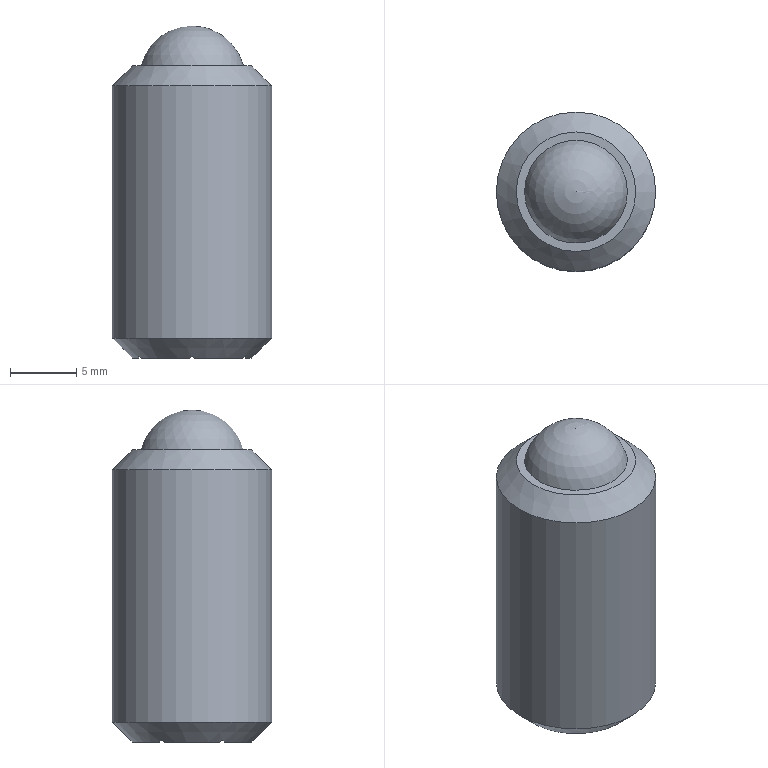Part | NX | features BZM12.00 2 | 1 solid | 18 faces | box 12 x 12 x 25 mm | volume 2052 mm3 | plane 14 | cone 2 | cylinder 1 | sphere 1 | commonest cylinder face diameters 12 x1
STEP:
#1=CARTESIAN_POINT('',(-101.,-82.938,-72.));
#2=VERTEX_POINT('',#1);
#3=CARTESIAN_POINT('',(-101.,-87.062,-72.));
#4=VERTEX_POINT('',#3);
#5=CARTESIAN_POINT('',(-101.,-82.691,-72.));
#6=DIRECTION('',(0.,-1.,0.));
#7=VECTOR('',#6,1000.);
#8=LINE('',#5,#7);
#9=EDGE_CURVE('',#2,#4,#8,.T.);
#10=ORIENTED_EDGE('',*,*,#9,.F.);
#11=CARTESIAN_POINT('',(-105.,-85.,-72.));
#12=DIRECTION('',(0.,0.,1.));
#13=DIRECTION('',(-1.,0.,0.));
#14=AXIS2_PLACEMENT_3D('',#11,#12,#13);
#15=CIRCLE('',#14,4.5);
#16=EDGE_CURVE('',#4,#2,#15,.T.);
#17=ORIENTED_EDGE('',*,*,#16,.F.);
#18=EDGE_LOOP('',(#10,#17));
#19=FACE_BOUND('',#18,.T.);
#20=CARTESIAN_POINT('',(-105.,-85.,-72.));
#21=DIRECTION('',(0.,0.,-1.));
#22=DIRECTION('',(-1.,0.,0.));
#23=AXIS2_PLACEMENT_3D('',#20,#21,#22);
#24=PLANE('',#23);
#25=ADVANCED_FACE('',(#19),#24,.T.);
#26=CARTESIAN_POINT('',(-104.785,-80.505,-72.));
#27=VERTEX_POINT('',#26);
#28=CARTESIAN_POINT('',(-101.215,-82.567,-72.));
#29=VERTEX_POINT('',#28);
#30=CARTESIAN_POINT('',(-105.,-80.381,-72.));
#31=DIRECTION('',(0.866,-0.5,0.));
#32=VECTOR('',#31,1000.);
#33=LINE('',#30,#32);
#34=EDGE_CURVE('',#27,#29,#33,.T.);
#35=ORIENTED_EDGE('',*,*,#34,.F.);
#36=CARTESIAN_POINT('',(-105.,-85.,-72.));
#37=DIRECTION('',(0.,0.,1.));
#38=DIRECTION('',(-1.,0.,0.));
#39=AXIS2_PLACEMENT_3D('',#36,#37,#38);
#40=CIRCLE('',#39,4.5);
#41=EDGE_CURVE('',#29,#27,#40,.T.);
#42=ORIENTED_EDGE('',*,*,#41,.F.);
#43=EDGE_LOOP('',(#35,#42));
#44=FACE_BOUND('',#43,.T.);
#45=CARTESIAN_POINT('',(-105.,-85.,-72.));
#46=DIRECTION('',(0.,0.,-1.));
#47=DIRECTION('',(-1.,0.,0.));
#48=AXIS2_PLACEMENT_3D('',#45,#46,#47);
#49=PLANE('',#48);
#50=ADVANCED_FACE('',(#44),#49,.T.);
#51=CARTESIAN_POINT('',(-108.785,-82.567,-72.));
#52=VERTEX_POINT('',#51);
#53=CARTESIAN_POINT('',(-105.215,-80.505,-72.));
#54=VERTEX_POINT('',#53);
#55=CARTESIAN_POINT('',(-109.,-82.691,-72.));
#56=DIRECTION('',(0.866,0.5,0.));
#57=VECTOR('',#56,1000.);
#58=LINE('',#55,#57);
#59=EDGE_CURVE('',#52,#54,#58,.T.);
#60=ORIENTED_EDGE('',*,*,#59,.F.);
#61=CARTESIAN_POINT('',(-105.,-85.,-72.));
#62=DIRECTION('',(0.,0.,1.));
#63=DIRECTION('',(-1.,0.,0.));
#64=AXIS2_PLACEMENT_3D('',#61,#62,#63);
#65=CIRCLE('',#64,4.5);
#66=EDGE_CURVE('',#54,#52,#65,.T.);
#67=ORIENTED_EDGE('',*,*,#66,.F.);
#68=EDGE_LOOP('',(#60,#67));
#69=FACE_BOUND('',#68,.T.);
#70=CARTESIAN_POINT('',(-105.,-85.,-72.));
#71=DIRECTION('',(0.,0.,-1.));
#72=DIRECTION('',(-1.,0.,0.));
#73=AXIS2_PLACEMENT_3D('',#70,#71,#72);
#74=PLANE('',#73);
#75=ADVANCED_FACE('',(#69),#74,.T.);
#76=CARTESIAN_POINT('',(-109.,-87.062,-72.));
#77=VERTEX_POINT('',#76);
#78=CARTESIAN_POINT('',(-109.,-82.938,-72.));
#79=VERTEX_POINT('',#78);
#80=CARTESIAN_POINT('',(-109.,-87.309,-72.));
#81=DIRECTION('',(0.,1.,0.));
#82=VECTOR('',#81,1000.);
#83=LINE('',#80,#82);
#84=EDGE_CURVE('',#77,#79,#83,.T.);
#85=ORIENTED_EDGE('',*,*,#84,.F.);
#86=CARTESIAN_POINT('',(-105.,-85.,-72.));
#87=DIRECTION('',(0.,0.,1.));
#88=DIRECTION('',(-1.,0.,0.));
#89=AXIS2_PLACEMENT_3D('',#86,#87,#88);
#90=CIRCLE('',#89,4.5);
#91=EDGE_CURVE('',#79,#77,#90,.T.);
#92=ORIENTED_EDGE('',*,*,#91,.F.);
#93=EDGE_LOOP('',(#85,#92));
#94=FACE_BOUND('',#93,.T.);
#95=CARTESIAN_POINT('',(-105.,-85.,-72.));
#96=DIRECTION('',(0.,0.,-1.));
#97=DIRECTION('',(-1.,0.,0.));
#98=AXIS2_PLACEMENT_3D('',#95,#96,#97);
#99=PLANE('',#98);
#100=ADVANCED_FACE('',(#94),#99,.T.);
#101=CARTESIAN_POINT('',(-105.215,-89.495,-72.));
#102=VERTEX_POINT('',#101);
#103=CARTESIAN_POINT('',(-108.785,-87.433,-72.));
#104=VERTEX_POINT('',#103);
#105=CARTESIAN_POINT('',(-105.,-89.619,-72.));
#106=DIRECTION('',(-0.866,0.5,0.));
#107=VECTOR('',#106,1000.);
#108=LINE('',#105,#107);
#109=EDGE_CURVE('',#102,#104,#108,.T.);
#110=ORIENTED_EDGE('',*,*,#109,.F.);
#111=CARTESIAN_POINT('',(-105.,-85.,-72.));
#112=DIRECTION('',(0.,0.,1.));
#113=DIRECTION('',(-1.,0.,0.));
#114=AXIS2_PLACEMENT_3D('',#111,#112,#113);
#115=CIRCLE('',#114,4.5);
#116=EDGE_CURVE('',#104,#102,#115,.T.);
#117=ORIENTED_EDGE('',*,*,#116,.F.);
#118=EDGE_LOOP('',(#110,#117));
#119=FACE_BOUND('',#118,.T.);
#120=CARTESIAN_POINT('',(-105.,-85.,-72.));
#121=DIRECTION('',(0.,0.,-1.));
#122=DIRECTION('',(-1.,0.,0.));
#123=AXIS2_PLACEMENT_3D('',#120,#121,#122);
#124=PLANE('',#123);
#125=ADVANCED_FACE('',(#119),#124,.T.);
#126=CARTESIAN_POINT('',(-101.215,-87.433,-72.));
#127=VERTEX_POINT('',#126);
#128=CARTESIAN_POINT('',(-104.785,-89.495,-72.));
#129=VERTEX_POINT('',#128);
#130=CARTESIAN_POINT('',(-101.,-87.309,-72.));
#131=DIRECTION('',(-0.866,-0.5,0.));
#132=VECTOR('',#131,1000.);
#133=LINE('',#130,#132);
#134=EDGE_CURVE('',#127,#129,#133,.T.);
#135=ORIENTED_EDGE('',*,*,#134,.F.);
#136=CARTESIAN_POINT('',(-105.,-85.,-72.));
#137=DIRECTION('',(0.,0.,1.));
#138=DIRECTION('',(-1.,0.,0.));
#139=AXIS2_PLACEMENT_3D('',#136,#137,#138);
#140=CIRCLE('',#139,4.5);
#141=EDGE_CURVE('',#129,#127,#140,.T.);
#142=ORIENTED_EDGE('',*,*,#141,.F.);
#143=EDGE_LOOP('',(#135,#142));
#144=FACE_BOUND('',#143,.T.);
#145=CARTESIAN_POINT('',(-105.,-85.,-72.));
#146=DIRECTION('',(0.,0.,-1.));
#147=DIRECTION('',(-1.,0.,0.));
#148=AXIS2_PLACEMENT_3D('',#145,#146,#147);
#149=PLANE('',#148);
#150=ADVANCED_FACE('',(#144),#149,.T.);
#151=CARTESIAN_POINT('',(-100.5,-85.,-50.));
#152=VERTEX_POINT('',#151);
#153=CARTESIAN_POINT('',(-105.,-85.,-50.));
#154=DIRECTION('',(0.,0.,-1.));
#155=DIRECTION('',(1.,0.,0.));
#156=AXIS2_PLACEMENT_3D('',#153,#154,#155);
#157=CIRCLE('',#156,4.5);
#158=EDGE_CURVE('',#152,#152,#157,.T.);
#159=ORIENTED_EDGE('',*,*,#158,.F.);
#160=EDGE_LOOP('',(#159));
#161=FACE_BOUND('',#160,.T.);
#162=CARTESIAN_POINT('',(-101.127,-85.,-50.));
#163=VERTEX_POINT('',#162);
#164=CARTESIAN_POINT('',(-105.,-85.,-50.));
#165=DIRECTION('',(0.,0.,-1.));
#166=DIRECTION('',(1.,0.,0.));
#167=AXIS2_PLACEMENT_3D('',#164,#165,#166);
#168=CIRCLE('',#167,3.873);
#169=EDGE_CURVE('',#163,#163,#168,.T.);
#170=ORIENTED_EDGE('',*,*,#169,.T.);
#171=EDGE_LOOP('',(#170));
#172=FACE_BOUND('',#171,.T.);
#173=CARTESIAN_POINT('',(-105.,-85.,-50.));
#174=DIRECTION('',(0.,0.,1.));
#175=DIRECTION('',(1.,0.,0.));
#176=AXIS2_PLACEMENT_3D('',#173,#174,#175);
#177=PLANE('',#176);
#178=ADVANCED_FACE('',(#161,#172),#177,.T.);
#179=CARTESIAN_POINT('',(-111.,-85.,-70.5));
#180=VERTEX_POINT('',#179);
#181=CARTESIAN_POINT('',(-105.,-85.,-70.5));
#182=DIRECTION('',(0.,0.,1.));
#183=DIRECTION('',(-1.,0.,0.));
#184=AXIS2_PLACEMENT_3D('',#181,#182,#183);
#185=CIRCLE('',#184,6.);
#186=EDGE_CURVE('',#180,#180,#185,.F.);
#187=ORIENTED_EDGE('',*,*,#186,.F.);
#188=EDGE_LOOP('',(#187));
#189=FACE_BOUND('',#188,.T.);
#190=CARTESIAN_POINT('',(-99.,-85.,-51.5));
#191=VERTEX_POINT('',#190);
#192=CARTESIAN_POINT('',(-105.,-85.,-51.5));
#193=DIRECTION('',(0.,0.,-1.));
#194=DIRECTION('',(1.,0.,0.));
#195=AXIS2_PLACEMENT_3D('',#192,#193,#194);
#196=CIRCLE('',#195,6.);
#197=EDGE_CURVE('',#191,#191,#196,.F.);
#198=ORIENTED_EDGE('',*,*,#197,.F.);
#199=EDGE_LOOP('',(#198));
#200=FACE_BOUND('',#199,.T.);
#201=CARTESIAN_POINT('',(-105.,-85.,-50.));
#202=DIRECTION('',(0.,0.,-1.));
#203=DIRECTION('',(1.,0.,0.));
#204=AXIS2_PLACEMENT_3D('',#201,#202,#203);
#205=CYLINDRICAL_SURFACE('',#204,6.);
#206=ADVANCED_FACE('',(#189,#200),#205,.T.);
#207=CARTESIAN_POINT('',(-105.,-80.381,-64.));
#208=VERTEX_POINT('',#207);
#209=CARTESIAN_POINT('',(-105.,-80.381,-71.881));
#210=VERTEX_POINT('',#209);
#211=CARTESIAN_POINT('',(-105.,-80.381,-72.));
#212=DIRECTION('',(0.,0.,1.));
#213=VECTOR('',#212,1000.);
#214=LINE('',#211,#213);
#215=EDGE_CURVE('',#208,#210,#214,.F.);
#216=ORIENTED_EDGE('',*,*,#215,.F.);
#217=CARTESIAN_POINT('',(-109.,-82.691,-64.));
#218=VERTEX_POINT('',#217);
#219=CARTESIAN_POINT('',(-109.,-82.691,-64.));
#220=DIRECTION('',(0.866,0.5,0.));
#221=VECTOR('',#220,1000.);
#222=LINE('',#219,#221);
#223=EDGE_CURVE('',#208,#218,#222,.F.);
#224=ORIENTED_EDGE('',*,*,#223,.T.);
#225=CARTESIAN_POINT('',(-109.,-82.691,-71.881));
#226=VERTEX_POINT('',#225);
#227=CARTESIAN_POINT('',(-109.,-82.691,-72.));
#228=DIRECTION('',(0.,0.,1.));
#229=VECTOR('',#228,1000.);
#230=LINE('',#227,#229);
#231=EDGE_CURVE('',#218,#226,#230,.F.);
#232=ORIENTED_EDGE('',*,*,#231,.T.);
#233=CARTESIAN_POINT('',(-108.785,-82.567,-72.));
#234=CARTESIAN_POINT('',(-108.858,-82.608,-71.962));
#235=CARTESIAN_POINT('',(-108.929,-82.65,-71.922));
#236=CARTESIAN_POINT('',(-109.,-82.691,-71.881));
#237=B_SPLINE_CURVE_WITH_KNOTS('',3,(#233,#234,#235,#236),.UNSPECIFIED.,.F.,.F.,(4,4),(0.,0.0002749),.UNSPECIFIED.);
#238=EDGE_CURVE('',#52,#226,#237,.T.);
#239=ORIENTED_EDGE('',*,*,#238,.F.);
#240=ORIENTED_EDGE('',*,*,#59,.T.);
#241=CARTESIAN_POINT('',(-105.,-80.381,-71.881));
#242=CARTESIAN_POINT('',(-105.071,-80.422,-71.922));
#243=CARTESIAN_POINT('',(-105.142,-80.463,-71.962));
#244=CARTESIAN_POINT('',(-105.215,-80.505,-72.));
#245=B_SPLINE_CURVE_WITH_KNOTS('',3,(#241,#242,#243,#244),.UNSPECIFIED.,.F.,.F.,(4,4),(0.,0.0002749),.UNSPECIFIED.);
#246=EDGE_CURVE('',#210,#54,#245,.T.);
#247=ORIENTED_EDGE('',*,*,#246,.F.);
#248=EDGE_LOOP('',(#216,#224,#232,#239,#240,#247));
#249=FACE_BOUND('',#248,.T.);
#250=CARTESIAN_POINT('',(-107.,-81.536,-68.));
#251=DIRECTION('',(-0.5,0.866,0.));
#252=DIRECTION('',(0.866,0.5,0.));
#253=AXIS2_PLACEMENT_3D('',#250,#251,#252);
#254=PLANE('',#253);
#255=ADVANCED_FACE('',(#249),#254,.F.);
#256=ORIENTED_EDGE('',*,*,#231,.F.);
#257=CARTESIAN_POINT('',(-109.,-87.309,-64.));
#258=VERTEX_POINT('',#257);
#259=CARTESIAN_POINT('',(-109.,-87.309,-64.));
#260=DIRECTION('',(0.,1.,0.));
#261=VECTOR('',#260,1000.);
#262=LINE('',#259,#261);
#263=EDGE_CURVE('',#218,#258,#262,.F.);
#264=ORIENTED_EDGE('',*,*,#263,.T.);
#265=CARTESIAN_POINT('',(-109.,-87.309,-71.881));
#266=VERTEX_POINT('',#265);
#267=CARTESIAN_POINT('',(-109.,-87.309,-72.));
#268=DIRECTION('',(0.,0.,1.));
#269=VECTOR('',#268,1000.);
#270=LINE('',#267,#269);
#271=EDGE_CURVE('',#258,#266,#270,.F.);
#272=ORIENTED_EDGE('',*,*,#271,.T.);
#273=CARTESIAN_POINT('',(-109.,-87.062,-72.));
#274=CARTESIAN_POINT('',(-109.,-87.145,-71.962));
#275=CARTESIAN_POINT('',(-109.,-87.227,-71.922));
#276=CARTESIAN_POINT('',(-109.,-87.309,-71.881));
#277=B_SPLINE_CURVE_WITH_KNOTS('',3,(#273,#274,#275,#276),.UNSPECIFIED.,.F.,.F.,(4,4),(0.,0.0002749),.UNSPECIFIED.);
#278=EDGE_CURVE('',#77,#266,#277,.T.);
#279=ORIENTED_EDGE('',*,*,#278,.F.);
#280=ORIENTED_EDGE('',*,*,#84,.T.);
#281=CARTESIAN_POINT('',(-109.,-82.691,-71.881));
#282=CARTESIAN_POINT('',(-109.,-82.773,-71.922));
#283=CARTESIAN_POINT('',(-109.,-82.855,-71.962));
#284=CARTESIAN_POINT('',(-109.,-82.938,-72.));
#285=B_SPLINE_CURVE_WITH_KNOTS('',3,(#281,#282,#283,#284),.UNSPECIFIED.,.F.,.F.,(4,4),(0.,0.0002749),.UNSPECIFIED.);
#286=EDGE_CURVE('',#226,#79,#285,.T.);
#287=ORIENTED_EDGE('',*,*,#286,.F.);
#288=EDGE_LOOP('',(#256,#264,#272,#279,#280,#287));
#289=FACE_BOUND('',#288,.T.);
#290=CARTESIAN_POINT('',(-109.,-85.,-68.));
#291=DIRECTION('',(-1.,0.,0.));
#292=DIRECTION('',(0.,0.,1.));
#293=AXIS2_PLACEMENT_3D('',#290,#291,#292);
#294=PLANE('',#293);
#295=ADVANCED_FACE('',(#289),#294,.F.);
#296=ORIENTED_EDGE('',*,*,#271,.F.);
#297=CARTESIAN_POINT('',(-105.,-89.619,-64.));
#298=VERTEX_POINT('',#297);
#299=CARTESIAN_POINT('',(-105.,-89.619,-64.));
#300=DIRECTION('',(-0.866,0.5,0.));
#301=VECTOR('',#300,1000.);
#302=LINE('',#299,#301);
#303=EDGE_CURVE('',#258,#298,#302,.F.);
#304=ORIENTED_EDGE('',*,*,#303,.T.);
#305=CARTESIAN_POINT('',(-105.,-89.619,-71.881));
#306=VERTEX_POINT('',#305);
#307=CARTESIAN_POINT('',(-105.,-89.619,-72.));
#308=DIRECTION('',(0.,0.,1.));
#309=VECTOR('',#308,1000.);
#310=LINE('',#307,#309);
#311=EDGE_CURVE('',#298,#306,#310,.F.);
#312=ORIENTED_EDGE('',*,*,#311,.T.);
#313=CARTESIAN_POINT('',(-105.215,-89.495,-72.));
#314=CARTESIAN_POINT('',(-105.142,-89.537,-71.962));
#315=CARTESIAN_POINT('',(-105.071,-89.578,-71.922));
#316=CARTESIAN_POINT('',(-105.,-89.619,-71.881));
#317=B_SPLINE_CURVE_WITH_KNOTS('',3,(#313,#314,#315,#316),.UNSPECIFIED.,.F.,.F.,(4,4),(0.,0.0002749),.UNSPECIFIED.);
#318=EDGE_CURVE('',#102,#306,#317,.T.);
#319=ORIENTED_EDGE('',*,*,#318,.F.);
#320=ORIENTED_EDGE('',*,*,#109,.T.);
#321=CARTESIAN_POINT('',(-109.,-87.309,-71.881));
#322=CARTESIAN_POINT('',(-108.929,-87.35,-71.922));
#323=CARTESIAN_POINT('',(-108.858,-87.392,-71.962));
#324=CARTESIAN_POINT('',(-108.785,-87.433,-72.));
#325=B_SPLINE_CURVE_WITH_KNOTS('',3,(#321,#322,#323,#324),.UNSPECIFIED.,.F.,.F.,(4,4),(0.,0.0002749),.UNSPECIFIED.);
#326=EDGE_CURVE('',#266,#104,#325,.T.);
#327=ORIENTED_EDGE('',*,*,#326,.F.);
#328=EDGE_LOOP('',(#296,#304,#312,#319,#320,#327));
#329=FACE_BOUND('',#328,.T.);
#330=CARTESIAN_POINT('',(-107.,-88.464,-68.));
#331=DIRECTION('',(-0.5,-0.866,0.));
#332=DIRECTION('',(-0.866,0.5,0.));
#333=AXIS2_PLACEMENT_3D('',#330,#331,#332);
#334=PLANE('',#333);
#335=ADVANCED_FACE('',(#329),#334,.F.);
#336=ORIENTED_EDGE('',*,*,#311,.F.);
#337=CARTESIAN_POINT('',(-101.,-87.309,-64.));
#338=VERTEX_POINT('',#337);
#339=CARTESIAN_POINT('',(-101.,-87.309,-64.));
#340=DIRECTION('',(-0.866,-0.5,0.));
#341=VECTOR('',#340,1000.);
#342=LINE('',#339,#341);
#343=EDGE_CURVE('',#298,#338,#342,.F.);
#344=ORIENTED_EDGE('',*,*,#343,.T.);
#345=CARTESIAN_POINT('',(-101.,-87.309,-71.881));
#346=VERTEX_POINT('',#345);
#347=CARTESIAN_POINT('',(-101.,-87.309,-72.));
#348=DIRECTION('',(0.,0.,1.));
#349=VECTOR('',#348,1000.);
#350=LINE('',#347,#349);
#351=EDGE_CURVE('',#338,#346,#350,.F.);
#352=ORIENTED_EDGE('',*,*,#351,.T.);
#353=CARTESIAN_POINT('',(-101.215,-87.433,-72.));
#354=CARTESIAN_POINT('',(-101.142,-87.392,-71.962));
#355=CARTESIAN_POINT('',(-101.071,-87.35,-71.922));
#356=CARTESIAN_POINT('',(-101.,-87.309,-71.881));
#357=B_SPLINE_CURVE_WITH_KNOTS('',3,(#353,#354,#355,#356),.UNSPECIFIED.,.F.,.F.,(4,4),(0.,0.0002749),.UNSPECIFIED.);
#358=EDGE_CURVE('',#127,#346,#357,.T.);
#359=ORIENTED_EDGE('',*,*,#358,.F.);
#360=ORIENTED_EDGE('',*,*,#134,.T.);
#361=CARTESIAN_POINT('',(-105.,-89.619,-71.881));
#362=CARTESIAN_POINT('',(-104.929,-89.578,-71.922));
#363=CARTESIAN_POINT('',(-104.858,-89.537,-71.962));
#364=CARTESIAN_POINT('',(-104.785,-89.495,-72.));
#365=B_SPLINE_CURVE_WITH_KNOTS('',3,(#361,#362,#363,#364),.UNSPECIFIED.,.F.,.F.,(4,4),(0.,0.0002749),.UNSPECIFIED.);
#366=EDGE_CURVE('',#306,#129,#365,.T.);
#367=ORIENTED_EDGE('',*,*,#366,.F.);
#368=EDGE_LOOP('',(#336,#344,#352,#359,#360,#367));
#369=FACE_BOUND('',#368,.T.);
#370=CARTESIAN_POINT('',(-103.,-88.464,-68.));
#371=DIRECTION('',(0.5,-0.866,0.));
#372=DIRECTION('',(-0.866,-0.5,0.));
#373=AXIS2_PLACEMENT_3D('',#370,#371,#372);
#374=PLANE('',#373);
#375=ADVANCED_FACE('',(#369),#374,.F.);
#376=ORIENTED_EDGE('',*,*,#9,.T.);
#377=CARTESIAN_POINT('',(-101.,-87.309,-71.881));
#378=CARTESIAN_POINT('',(-101.,-87.227,-71.922));
#379=CARTESIAN_POINT('',(-101.,-87.145,-71.962));
#380=CARTESIAN_POINT('',(-101.,-87.062,-72.));
#381=B_SPLINE_CURVE_WITH_KNOTS('',3,(#377,#378,#379,#380),.UNSPECIFIED.,.F.,.F.,(4,4),(0.,0.0002749),.UNSPECIFIED.);
#382=EDGE_CURVE('',#346,#4,#381,.T.);
#383=ORIENTED_EDGE('',*,*,#382,.F.);
#384=ORIENTED_EDGE('',*,*,#351,.F.);
#385=CARTESIAN_POINT('',(-101.,-82.691,-64.));
#386=VERTEX_POINT('',#385);
#387=CARTESIAN_POINT('',(-101.,-82.691,-64.));
#388=DIRECTION('',(0.,-1.,0.));
#389=VECTOR('',#388,1000.);
#390=LINE('',#387,#389);
#391=EDGE_CURVE('',#338,#386,#390,.F.);
#392=ORIENTED_EDGE('',*,*,#391,.T.);
#393=CARTESIAN_POINT('',(-101.,-82.691,-71.881));
#394=VERTEX_POINT('',#393);
#395=CARTESIAN_POINT('',(-101.,-82.691,-72.));
#396=DIRECTION('',(0.,0.,1.));
#397=VECTOR('',#396,1000.);
#398=LINE('',#395,#397);
#399=EDGE_CURVE('',#386,#394,#398,.F.);
#400=ORIENTED_EDGE('',*,*,#399,.T.);
#401=CARTESIAN_POINT('',(-101.,-82.938,-72.));
#402=CARTESIAN_POINT('',(-101.,-82.855,-71.962));
#403=CARTESIAN_POINT('',(-101.,-82.773,-71.922));
#404=CARTESIAN_POINT('',(-101.,-82.691,-71.881));
#405=B_SPLINE_CURVE_WITH_KNOTS('',3,(#401,#402,#403,#404),.UNSPECIFIED.,.F.,.F.,(4,4),(0.,0.0002749),.UNSPECIFIED.);
#406=EDGE_CURVE('',#2,#394,#405,.T.);
#407=ORIENTED_EDGE('',*,*,#406,.F.);
#408=EDGE_LOOP('',(#376,#383,#384,#392,#400,#407));
#409=FACE_BOUND('',#408,.T.);
#410=CARTESIAN_POINT('',(-101.,-85.,-68.));
#411=DIRECTION('',(1.,0.,0.));
#412=DIRECTION('',(0.,0.,-1.));
#413=AXIS2_PLACEMENT_3D('',#410,#411,#412);
#414=PLANE('',#413);
#415=ADVANCED_FACE('',(#409),#414,.F.);
#416=ORIENTED_EDGE('',*,*,#399,.F.);
#417=CARTESIAN_POINT('',(-105.,-80.381,-64.));
#418=DIRECTION('',(0.866,-0.5,0.));
#419=VECTOR('',#418,1000.);
#420=LINE('',#417,#419);
#421=EDGE_CURVE('',#386,#208,#420,.F.);
#422=ORIENTED_EDGE('',*,*,#421,.T.);
#423=ORIENTED_EDGE('',*,*,#215,.T.);
#424=CARTESIAN_POINT('',(-104.785,-80.505,-72.));
#425=CARTESIAN_POINT('',(-104.858,-80.463,-71.962));
#426=CARTESIAN_POINT('',(-104.929,-80.422,-71.922));
#427=CARTESIAN_POINT('',(-105.,-80.381,-71.881));
#428=B_SPLINE_CURVE_WITH_KNOTS('',3,(#424,#425,#426,#427),.UNSPECIFIED.,.F.,.F.,(4,4),(0.,0.0002749),.UNSPECIFIED.);
#429=EDGE_CURVE('',#27,#210,#428,.T.);
#430=ORIENTED_EDGE('',*,*,#429,.F.);
#431=ORIENTED_EDGE('',*,*,#34,.T.);
#432=CARTESIAN_POINT('',(-101.,-82.691,-71.881));
#433=CARTESIAN_POINT('',(-101.071,-82.65,-71.922));
#434=CARTESIAN_POINT('',(-101.142,-82.608,-71.962));
#435=CARTESIAN_POINT('',(-101.215,-82.567,-72.));
#436=B_SPLINE_CURVE_WITH_KNOTS('',3,(#432,#433,#434,#435),.UNSPECIFIED.,.F.,.F.,(4,4),(0.,0.0002749),.UNSPECIFIED.);
#437=EDGE_CURVE('',#394,#29,#436,.T.);
#438=ORIENTED_EDGE('',*,*,#437,.F.);
#439=EDGE_LOOP('',(#416,#422,#423,#430,#431,#438));
#440=FACE_BOUND('',#439,.T.);
#441=CARTESIAN_POINT('',(-103.,-81.536,-68.));
#442=DIRECTION('',(0.5,0.866,0.));
#443=DIRECTION('',(0.866,-0.5,0.));
#444=AXIS2_PLACEMENT_3D('',#441,#442,#443);
#445=PLANE('',#444);
#446=ADVANCED_FACE('',(#440),#445,.F.);
#447=ORIENTED_EDGE('',*,*,#263,.F.);
#448=ORIENTED_EDGE('',*,*,#223,.F.);
#449=ORIENTED_EDGE('',*,*,#421,.F.);
#450=ORIENTED_EDGE('',*,*,#391,.F.);
#451=ORIENTED_EDGE('',*,*,#343,.F.);
#452=ORIENTED_EDGE('',*,*,#303,.F.);
#453=EDGE_LOOP('',(#447,#448,#449,#450,#451,#452));
#454=FACE_BOUND('',#453,.T.);
#455=CARTESIAN_POINT('',(-105.,-85.,-64.));
#456=DIRECTION('',(0.,0.,1.));
#457=DIRECTION('',(1.,0.,0.));
#458=AXIS2_PLACEMENT_3D('',#455,#456,#457);
#459=PLANE('',#458);
#460=ADVANCED_FACE('',(#454),#459,.F.);
#461=ORIENTED_EDGE('',*,*,#169,.F.);
#462=EDGE_LOOP('',(#461));
#463=FACE_BOUND('',#462,.T.);
#464=CARTESIAN_POINT('',(-105.,-85.,-51.));
#465=DIRECTION('',(0.,0.,1.));
#466=DIRECTION('',(1.,0.,0.));
#467=AXIS2_PLACEMENT_3D('',#464,#465,#466);
#468=SPHERICAL_SURFACE('',#467,4.);
#469=ADVANCED_FACE('',(#463),#468,.T.);
#470=ORIENTED_EDGE('',*,*,#406,.T.);
#471=ORIENTED_EDGE('',*,*,#437,.T.);
#472=ORIENTED_EDGE('',*,*,#41,.T.);
#473=ORIENTED_EDGE('',*,*,#429,.T.);
#474=ORIENTED_EDGE('',*,*,#246,.T.);
#475=ORIENTED_EDGE('',*,*,#66,.T.);
#476=ORIENTED_EDGE('',*,*,#238,.T.);
#477=ORIENTED_EDGE('',*,*,#286,.T.);
#478=ORIENTED_EDGE('',*,*,#91,.T.);
#479=ORIENTED_EDGE('',*,*,#278,.T.);
#480=ORIENTED_EDGE('',*,*,#326,.T.);
#481=ORIENTED_EDGE('',*,*,#116,.T.);
#482=ORIENTED_EDGE('',*,*,#318,.T.);
#483=ORIENTED_EDGE('',*,*,#366,.T.);
#484=ORIENTED_EDGE('',*,*,#141,.T.);
#485=ORIENTED_EDGE('',*,*,#358,.T.);
#486=ORIENTED_EDGE('',*,*,#382,.T.);
#487=ORIENTED_EDGE('',*,*,#16,.T.);
#488=EDGE_LOOP('',(#470,#471,#472,#473,#474,#475,#476,#477,#478,#479,#480,#481,#482,#483,#484,#485,#486,#487));
#489=FACE_BOUND('',#488,.T.);
#490=ORIENTED_EDGE('',*,*,#186,.T.);
#491=EDGE_LOOP('',(#490));
#492=FACE_BOUND('',#491,.T.);
#493=CARTESIAN_POINT('',(-105.,-85.,-70.5));
#494=DIRECTION('',(0.,0.,1.));
#495=DIRECTION('',(1.,0.,0.));
#496=AXIS2_PLACEMENT_3D('',#493,#494,#495);
#497=CONICAL_SURFACE('',#496,6.,0.7854);
#498=ADVANCED_FACE('',(#489,#492),#497,.T.);
#499=ORIENTED_EDGE('',*,*,#158,.T.);
#500=EDGE_LOOP('',(#499));
#501=FACE_BOUND('',#500,.T.);
#502=ORIENTED_EDGE('',*,*,#197,.T.);
#503=EDGE_LOOP('',(#502));
#504=FACE_BOUND('',#503,.T.);
#505=CARTESIAN_POINT('',(-105.,-85.,-51.5));
#506=DIRECTION('',(0.,0.,-1.));
#507=DIRECTION('',(-1.,0.,0.));
#508=AXIS2_PLACEMENT_3D('',#505,#506,#507);
#509=CONICAL_SURFACE('',#508,6.,0.7854);
#510=ADVANCED_FACE('',(#501,#504),#509,.T.);
#511=CLOSED_SHELL('',(#25,#50,#75,#100,#125,#150,#178,#206,#255,#295,#335,#375,#415,#446,#460,#469,#498,#510));
#512=MANIFOLD_SOLID_BREP('',#511);
#513=(LENGTH_UNIT()NAMED_UNIT(*)SI_UNIT(.MILLI.,.METRE.));
#514=UNCERTAINTY_MEASURE_WITH_UNIT(LENGTH_MEASURE(0.0508),#513,'','');
#515=(NAMED_UNIT(*)PLANE_ANGLE_UNIT()SI_UNIT($,.RADIAN.));
#516=(NAMED_UNIT(*)SI_UNIT($,.STERADIAN.)SOLID_ANGLE_UNIT());
#517=(GEOMETRIC_REPRESENTATION_CONTEXT(3)GLOBAL_UNCERTAINTY_ASSIGNED_CONTEXT((#514))GLOBAL_UNIT_ASSIGNED_CONTEXT((#513,#515,#516))REPRESENTATION_CONTEXT('',''));
#518=ADVANCED_BREP_SHAPE_REPRESENTATION('',(#512),#517);